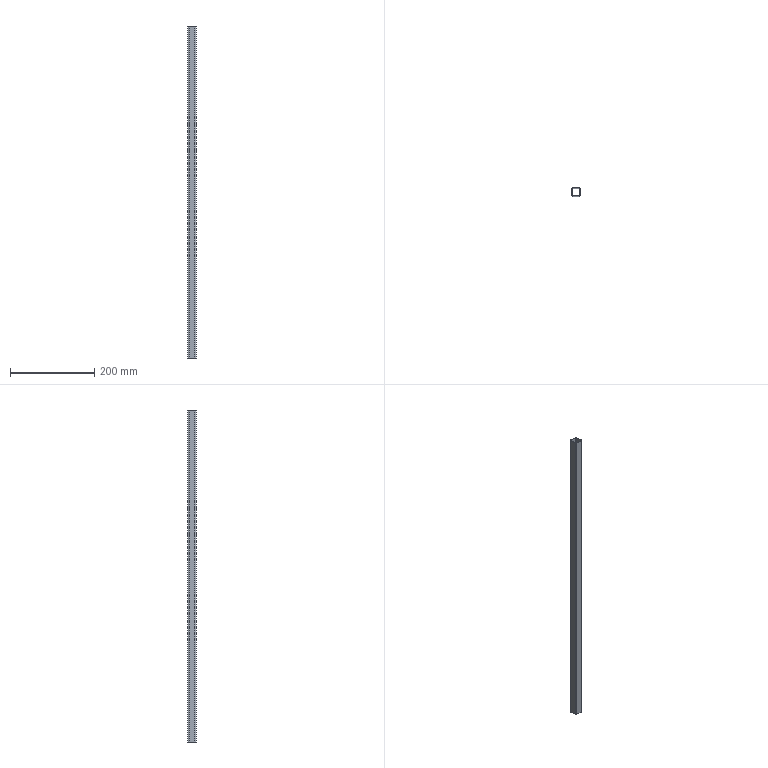Part | SolidWorks | features BaseBody 1 | 1 solid | 18 faces | box 20 x 20 x 786.319 mm | volume 67070 mm3 | plane 10 | cylinder 8 | commonest cylinder face diameters 3.6 x4 6 x4
STEP:
#1=CARTESIAN_POINT('',(7.,-8.8,0.));
#2=VERTEX_POINT('',#1);
#3=CARTESIAN_POINT('',(7.,-8.8,786.319));
#4=VERTEX_POINT('',#3);
#5=CARTESIAN_POINT('',(7.,-8.8,0.));
#6=DIRECTION('',(0.,0.,1.));
#7=VECTOR('',#6,1000.);
#8=LINE('',#5,#7);
#9=EDGE_CURVE('',#2,#4,#8,.T.);
#10=ORIENTED_EDGE('',*,*,#9,.F.);
#11=CARTESIAN_POINT('',(-7.,-8.8,0.));
#12=VERTEX_POINT('',#11);
#13=CARTESIAN_POINT('',(7.,-8.8,0.));
#14=DIRECTION('',(1.,0.,0.));
#15=VECTOR('',#14,1000.);
#16=LINE('',#13,#15);
#17=EDGE_CURVE('',#12,#2,#16,.T.);
#18=ORIENTED_EDGE('',*,*,#17,.F.);
#19=CARTESIAN_POINT('',(-7.,-8.8,786.319));
#20=VERTEX_POINT('',#19);
#21=CARTESIAN_POINT('',(-7.,-8.8,0.));
#22=DIRECTION('',(0.,0.,-1.));
#23=VECTOR('',#22,1000.);
#24=LINE('',#21,#23);
#25=EDGE_CURVE('',#20,#12,#24,.T.);
#26=ORIENTED_EDGE('',*,*,#25,.F.);
#27=CARTESIAN_POINT('',(7.,-8.8,786.319));
#28=DIRECTION('',(-1.,0.,0.));
#29=VECTOR('',#28,1000.);
#30=LINE('',#27,#29);
#31=EDGE_CURVE('',#4,#20,#30,.T.);
#32=ORIENTED_EDGE('',*,*,#31,.F.);
#33=EDGE_LOOP('',(#10,#18,#26,#32));
#34=FACE_OUTER_BOUND('',#33,.T.);
#35=CARTESIAN_POINT('',(7.,-8.8,0.));
#36=DIRECTION('',(0.,-1.,0.));
#37=DIRECTION('',(1.,0.,0.));
#38=AXIS2_PLACEMENT_3D('',#35,#36,#37);
#39=PLANE('',#38);
#40=ADVANCED_FACE('',(#34),#39,.F.);
#41=CARTESIAN_POINT('',(-8.8,-7.,786.319));
#42=VERTEX_POINT('',#41);
#43=CARTESIAN_POINT('',(-8.8,7.,786.319));
#44=VERTEX_POINT('',#43);
#45=CARTESIAN_POINT('',(-8.8,0.,786.319));
#46=DIRECTION('',(0.,1.,0.));
#47=VECTOR('',#46,1000.);
#48=LINE('',#45,#47);
#49=EDGE_CURVE('',#42,#44,#48,.T.);
#50=ORIENTED_EDGE('',*,*,#49,.T.);
#51=CARTESIAN_POINT('',(-7.,8.8,786.319));
#52=VERTEX_POINT('',#51);
#53=CARTESIAN_POINT('',(-7.,7.,786.319));
#54=DIRECTION('',(0.,0.,-1.));
#55=DIRECTION('',(1.,0.,0.));
#56=AXIS2_PLACEMENT_3D('',#53,#54,#55);
#57=CIRCLE('',#56,1.8);
#58=EDGE_CURVE('',#44,#52,#57,.T.);
#59=ORIENTED_EDGE('',*,*,#58,.T.);
#60=CARTESIAN_POINT('',(7.,8.8,786.319));
#61=VERTEX_POINT('',#60);
#62=CARTESIAN_POINT('',(0.,8.8,786.319));
#63=DIRECTION('',(1.,0.,0.));
#64=VECTOR('',#63,1000.);
#65=LINE('',#62,#64);
#66=EDGE_CURVE('',#52,#61,#65,.T.);
#67=ORIENTED_EDGE('',*,*,#66,.T.);
#68=CARTESIAN_POINT('',(8.8,7.,786.319));
#69=VERTEX_POINT('',#68);
#70=CARTESIAN_POINT('',(7.,7.,786.319));
#71=DIRECTION('',(0.,0.,-1.));
#72=DIRECTION('',(1.,0.,0.));
#73=AXIS2_PLACEMENT_3D('',#70,#71,#72);
#74=CIRCLE('',#73,1.8);
#75=EDGE_CURVE('',#61,#69,#74,.T.);
#76=ORIENTED_EDGE('',*,*,#75,.T.);
#77=CARTESIAN_POINT('',(8.8,-7.,786.319));
#78=VERTEX_POINT('',#77);
#79=CARTESIAN_POINT('',(8.8,0.,786.319));
#80=DIRECTION('',(0.,-1.,0.));
#81=VECTOR('',#80,1000.);
#82=LINE('',#79,#81);
#83=EDGE_CURVE('',#69,#78,#82,.T.);
#84=ORIENTED_EDGE('',*,*,#83,.T.);
#85=CARTESIAN_POINT('',(7.,-7.,786.319));
#86=DIRECTION('',(0.,0.,-1.));
#87=DIRECTION('',(1.,0.,0.));
#88=AXIS2_PLACEMENT_3D('',#85,#86,#87);
#89=CIRCLE('',#88,1.8);
#90=EDGE_CURVE('',#78,#4,#89,.T.);
#91=ORIENTED_EDGE('',*,*,#90,.T.);
#92=ORIENTED_EDGE('',*,*,#31,.T.);
#93=CARTESIAN_POINT('',(-7.,-7.,786.319));
#94=DIRECTION('',(0.,0.,-1.));
#95=DIRECTION('',(1.,0.,0.));
#96=AXIS2_PLACEMENT_3D('',#93,#94,#95);
#97=CIRCLE('',#96,1.8);
#98=EDGE_CURVE('',#20,#42,#97,.T.);
#99=ORIENTED_EDGE('',*,*,#98,.T.);
#100=EDGE_LOOP('',(#50,#59,#67,#76,#84,#91,#92,#99));
#101=FACE_BOUND('',#100,.T.);
#102=CARTESIAN_POINT('',(7.,10.,786.319));
#103=VERTEX_POINT('',#102);
#104=CARTESIAN_POINT('',(-7.,10.,786.319));
#105=VERTEX_POINT('',#104);
#106=CARTESIAN_POINT('',(0.,10.,786.319));
#107=DIRECTION('',(-1.,0.,0.));
#108=VECTOR('',#107,1000.);
#109=LINE('',#106,#108);
#110=EDGE_CURVE('',#103,#105,#109,.T.);
#111=ORIENTED_EDGE('',*,*,#110,.T.);
#112=CARTESIAN_POINT('',(-10.,7.,786.319));
#113=VERTEX_POINT('',#112);
#114=CARTESIAN_POINT('',(-7.,7.,786.319));
#115=DIRECTION('',(0.,0.,1.));
#116=DIRECTION('',(1.,0.,0.));
#117=AXIS2_PLACEMENT_3D('',#114,#115,#116);
#118=CIRCLE('',#117,3.);
#119=EDGE_CURVE('',#105,#113,#118,.T.);
#120=ORIENTED_EDGE('',*,*,#119,.T.);
#121=CARTESIAN_POINT('',(-10.,-7.,786.319));
#122=VERTEX_POINT('',#121);
#123=CARTESIAN_POINT('',(-10.,0.,786.319));
#124=DIRECTION('',(0.,-1.,0.));
#125=VECTOR('',#124,1000.);
#126=LINE('',#123,#125);
#127=EDGE_CURVE('',#113,#122,#126,.T.);
#128=ORIENTED_EDGE('',*,*,#127,.T.);
#129=CARTESIAN_POINT('',(-7.,-10.,786.319));
#130=VERTEX_POINT('',#129);
#131=CARTESIAN_POINT('',(-7.,-7.,786.319));
#132=DIRECTION('',(0.,0.,1.));
#133=DIRECTION('',(1.,0.,0.));
#134=AXIS2_PLACEMENT_3D('',#131,#132,#133);
#135=CIRCLE('',#134,3.);
#136=EDGE_CURVE('',#122,#130,#135,.T.);
#137=ORIENTED_EDGE('',*,*,#136,.T.);
#138=CARTESIAN_POINT('',(7.,-10.,786.319));
#139=VERTEX_POINT('',#138);
#140=CARTESIAN_POINT('',(0.,-10.,786.319));
#141=DIRECTION('',(1.,0.,0.));
#142=VECTOR('',#141,1000.);
#143=LINE('',#140,#142);
#144=EDGE_CURVE('',#130,#139,#143,.T.);
#145=ORIENTED_EDGE('',*,*,#144,.T.);
#146=CARTESIAN_POINT('',(10.,-7.,786.319));
#147=VERTEX_POINT('',#146);
#148=CARTESIAN_POINT('',(7.,-7.,786.319));
#149=DIRECTION('',(0.,0.,1.));
#150=DIRECTION('',(1.,0.,0.));
#151=AXIS2_PLACEMENT_3D('',#148,#149,#150);
#152=CIRCLE('',#151,3.);
#153=EDGE_CURVE('',#139,#147,#152,.T.);
#154=ORIENTED_EDGE('',*,*,#153,.T.);
#155=CARTESIAN_POINT('',(10.,7.,786.319));
#156=VERTEX_POINT('',#155);
#157=CARTESIAN_POINT('',(10.,0.,786.319));
#158=DIRECTION('',(0.,1.,0.));
#159=VECTOR('',#158,1000.);
#160=LINE('',#157,#159);
#161=EDGE_CURVE('',#147,#156,#160,.T.);
#162=ORIENTED_EDGE('',*,*,#161,.T.);
#163=CARTESIAN_POINT('',(7.,7.,786.319));
#164=DIRECTION('',(0.,0.,1.));
#165=DIRECTION('',(1.,0.,0.));
#166=AXIS2_PLACEMENT_3D('',#163,#164,#165);
#167=CIRCLE('',#166,3.);
#168=EDGE_CURVE('',#156,#103,#167,.T.);
#169=ORIENTED_EDGE('',*,*,#168,.T.);
#170=EDGE_LOOP('',(#111,#120,#128,#137,#145,#154,#162,#169));
#171=FACE_OUTER_BOUND('',#170,.T.);
#172=CARTESIAN_POINT('',(0.,0.,786.319));
#173=DIRECTION('',(0.,0.,1.));
#174=DIRECTION('',(1.,0.,0.));
#175=AXIS2_PLACEMENT_3D('',#172,#173,#174);
#176=PLANE('',#175);
#177=ADVANCED_FACE('',(#101,#171),#176,.T.);
#178=CARTESIAN_POINT('',(8.8,-7.,0.));
#179=VERTEX_POINT('',#178);
#180=CARTESIAN_POINT('',(8.8,-7.,0.));
#181=DIRECTION('',(0.,0.,1.));
#182=VECTOR('',#181,1000.);
#183=LINE('',#180,#182);
#184=EDGE_CURVE('',#179,#78,#183,.T.);
#185=ORIENTED_EDGE('',*,*,#184,.F.);
#186=CARTESIAN_POINT('',(7.,-7.,0.));
#187=DIRECTION('',(0.,0.,1.));
#188=DIRECTION('',(1.,0.,0.));
#189=AXIS2_PLACEMENT_3D('',#186,#187,#188);
#190=CIRCLE('',#189,1.8);
#191=EDGE_CURVE('',#2,#179,#190,.T.);
#192=ORIENTED_EDGE('',*,*,#191,.F.);
#193=ORIENTED_EDGE('',*,*,#9,.T.);
#194=ORIENTED_EDGE('',*,*,#90,.F.);
#195=EDGE_LOOP('',(#185,#192,#193,#194));
#196=FACE_OUTER_BOUND('',#195,.T.);
#197=CARTESIAN_POINT('',(7.,-7.,0.));
#198=DIRECTION('',(0.,0.,1.));
#199=DIRECTION('',(1.,0.,0.));
#200=AXIS2_PLACEMENT_3D('',#197,#198,#199);
#201=CYLINDRICAL_SURFACE('',#200,1.8);
#202=ADVANCED_FACE('',(#196),#201,.F.);
#203=CARTESIAN_POINT('',(-8.8,7.,0.));
#204=VERTEX_POINT('',#203);
#205=CARTESIAN_POINT('',(-7.,8.8,0.));
#206=VERTEX_POINT('',#205);
#207=CARTESIAN_POINT('',(-7.,7.,0.));
#208=DIRECTION('',(0.,0.,-1.));
#209=DIRECTION('',(1.,0.,0.));
#210=AXIS2_PLACEMENT_3D('',#207,#208,#209);
#211=CIRCLE('',#210,1.8);
#212=EDGE_CURVE('',#204,#206,#211,.T.);
#213=ORIENTED_EDGE('',*,*,#212,.F.);
#214=CARTESIAN_POINT('',(-8.8,-7.,0.));
#215=VERTEX_POINT('',#214);
#216=CARTESIAN_POINT('',(-8.8,0.,0.));
#217=DIRECTION('',(0.,1.,0.));
#218=VECTOR('',#217,1000.);
#219=LINE('',#216,#218);
#220=EDGE_CURVE('',#215,#204,#219,.T.);
#221=ORIENTED_EDGE('',*,*,#220,.F.);
#222=CARTESIAN_POINT('',(-7.,-7.,0.));
#223=DIRECTION('',(0.,0.,-1.));
#224=DIRECTION('',(1.,0.,0.));
#225=AXIS2_PLACEMENT_3D('',#222,#223,#224);
#226=CIRCLE('',#225,1.8);
#227=EDGE_CURVE('',#12,#215,#226,.T.);
#228=ORIENTED_EDGE('',*,*,#227,.F.);
#229=ORIENTED_EDGE('',*,*,#17,.T.);
#230=ORIENTED_EDGE('',*,*,#191,.T.);
#231=CARTESIAN_POINT('',(8.8,7.,0.));
#232=VERTEX_POINT('',#231);
#233=CARTESIAN_POINT('',(8.8,0.,0.));
#234=DIRECTION('',(0.,-1.,0.));
#235=VECTOR('',#234,1000.);
#236=LINE('',#233,#235);
#237=EDGE_CURVE('',#232,#179,#236,.T.);
#238=ORIENTED_EDGE('',*,*,#237,.F.);
#239=CARTESIAN_POINT('',(7.,8.8,0.));
#240=VERTEX_POINT('',#239);
#241=CARTESIAN_POINT('',(7.,7.,0.));
#242=DIRECTION('',(0.,0.,-1.));
#243=DIRECTION('',(1.,0.,0.));
#244=AXIS2_PLACEMENT_3D('',#241,#242,#243);
#245=CIRCLE('',#244,1.8);
#246=EDGE_CURVE('',#240,#232,#245,.T.);
#247=ORIENTED_EDGE('',*,*,#246,.F.);
#248=CARTESIAN_POINT('',(0.,8.8,0.));
#249=DIRECTION('',(1.,0.,0.));
#250=VECTOR('',#249,1000.);
#251=LINE('',#248,#250);
#252=EDGE_CURVE('',#206,#240,#251,.T.);
#253=ORIENTED_EDGE('',*,*,#252,.F.);
#254=EDGE_LOOP('',(#213,#221,#228,#229,#230,#238,#247,#253));
#255=FACE_BOUND('',#254,.T.);
#256=CARTESIAN_POINT('',(-7.,10.,0.));
#257=VERTEX_POINT('',#256);
#258=CARTESIAN_POINT('',(-10.,7.,0.));
#259=VERTEX_POINT('',#258);
#260=CARTESIAN_POINT('',(-7.,7.,0.));
#261=DIRECTION('',(0.,0.,1.));
#262=DIRECTION('',(1.,0.,0.));
#263=AXIS2_PLACEMENT_3D('',#260,#261,#262);
#264=CIRCLE('',#263,3.);
#265=EDGE_CURVE('',#257,#259,#264,.T.);
#266=ORIENTED_EDGE('',*,*,#265,.F.);
#267=CARTESIAN_POINT('',(7.,10.,0.));
#268=VERTEX_POINT('',#267);
#269=CARTESIAN_POINT('',(0.,10.,0.));
#270=DIRECTION('',(-1.,0.,0.));
#271=VECTOR('',#270,1000.);
#272=LINE('',#269,#271);
#273=EDGE_CURVE('',#268,#257,#272,.T.);
#274=ORIENTED_EDGE('',*,*,#273,.F.);
#275=CARTESIAN_POINT('',(10.,7.,0.));
#276=VERTEX_POINT('',#275);
#277=CARTESIAN_POINT('',(7.,7.,0.));
#278=DIRECTION('',(0.,0.,1.));
#279=DIRECTION('',(1.,0.,0.));
#280=AXIS2_PLACEMENT_3D('',#277,#278,#279);
#281=CIRCLE('',#280,3.);
#282=EDGE_CURVE('',#276,#268,#281,.T.);
#283=ORIENTED_EDGE('',*,*,#282,.F.);
#284=CARTESIAN_POINT('',(10.,-7.,0.));
#285=VERTEX_POINT('',#284);
#286=CARTESIAN_POINT('',(10.,0.,0.));
#287=DIRECTION('',(0.,1.,0.));
#288=VECTOR('',#287,1000.);
#289=LINE('',#286,#288);
#290=EDGE_CURVE('',#285,#276,#289,.T.);
#291=ORIENTED_EDGE('',*,*,#290,.F.);
#292=CARTESIAN_POINT('',(7.,-10.,0.));
#293=VERTEX_POINT('',#292);
#294=CARTESIAN_POINT('',(7.,-7.,0.));
#295=DIRECTION('',(0.,0.,1.));
#296=DIRECTION('',(1.,0.,0.));
#297=AXIS2_PLACEMENT_3D('',#294,#295,#296);
#298=CIRCLE('',#297,3.);
#299=EDGE_CURVE('',#293,#285,#298,.T.);
#300=ORIENTED_EDGE('',*,*,#299,.F.);
#301=CARTESIAN_POINT('',(-7.,-10.,0.));
#302=VERTEX_POINT('',#301);
#303=CARTESIAN_POINT('',(0.,-10.,0.));
#304=DIRECTION('',(1.,0.,0.));
#305=VECTOR('',#304,1000.);
#306=LINE('',#303,#305);
#307=EDGE_CURVE('',#302,#293,#306,.T.);
#308=ORIENTED_EDGE('',*,*,#307,.F.);
#309=CARTESIAN_POINT('',(-10.,-7.,0.));
#310=VERTEX_POINT('',#309);
#311=CARTESIAN_POINT('',(-7.,-7.,0.));
#312=DIRECTION('',(0.,0.,1.));
#313=DIRECTION('',(1.,0.,0.));
#314=AXIS2_PLACEMENT_3D('',#311,#312,#313);
#315=CIRCLE('',#314,3.);
#316=EDGE_CURVE('',#310,#302,#315,.T.);
#317=ORIENTED_EDGE('',*,*,#316,.F.);
#318=CARTESIAN_POINT('',(-10.,0.,0.));
#319=DIRECTION('',(0.,-1.,0.));
#320=VECTOR('',#319,1000.);
#321=LINE('',#318,#320);
#322=EDGE_CURVE('',#259,#310,#321,.T.);
#323=ORIENTED_EDGE('',*,*,#322,.F.);
#324=EDGE_LOOP('',(#266,#274,#283,#291,#300,#308,#317,#323));
#325=FACE_OUTER_BOUND('',#324,.T.);
#326=CARTESIAN_POINT('',(0.,0.,0.));
#327=DIRECTION('',(0.,0.,1.));
#328=DIRECTION('',(1.,0.,0.));
#329=AXIS2_PLACEMENT_3D('',#326,#327,#328);
#330=PLANE('',#329);
#331=ADVANCED_FACE('',(#255,#325),#330,.F.);
#332=ORIENTED_EDGE('',*,*,#25,.T.);
#333=ORIENTED_EDGE('',*,*,#227,.T.);
#334=CARTESIAN_POINT('',(-8.8,-7.,0.));
#335=DIRECTION('',(0.,0.,-1.));
#336=VECTOR('',#335,1000.);
#337=LINE('',#334,#336);
#338=EDGE_CURVE('',#42,#215,#337,.T.);
#339=ORIENTED_EDGE('',*,*,#338,.F.);
#340=ORIENTED_EDGE('',*,*,#98,.F.);
#341=EDGE_LOOP('',(#332,#333,#339,#340));
#342=FACE_OUTER_BOUND('',#341,.T.);
#343=CARTESIAN_POINT('',(-7.,-7.,0.));
#344=DIRECTION('',(0.,0.,1.));
#345=DIRECTION('',(1.,0.,0.));
#346=AXIS2_PLACEMENT_3D('',#343,#344,#345);
#347=CYLINDRICAL_SURFACE('',#346,1.8);
#348=ADVANCED_FACE('',(#342),#347,.F.);
#349=CARTESIAN_POINT('',(-8.8,7.,0.));
#350=DIRECTION('',(0.,0.,1.));
#351=VECTOR('',#350,1000.);
#352=LINE('',#349,#351);
#353=EDGE_CURVE('',#204,#44,#352,.T.);
#354=ORIENTED_EDGE('',*,*,#353,.F.);
#355=ORIENTED_EDGE('',*,*,#212,.T.);
#356=CARTESIAN_POINT('',(-7.,8.8,0.));
#357=DIRECTION('',(0.,0.,-1.));
#358=VECTOR('',#357,1000.);
#359=LINE('',#356,#358);
#360=EDGE_CURVE('',#52,#206,#359,.T.);
#361=ORIENTED_EDGE('',*,*,#360,.F.);
#362=ORIENTED_EDGE('',*,*,#58,.F.);
#363=EDGE_LOOP('',(#354,#355,#361,#362));
#364=FACE_OUTER_BOUND('',#363,.T.);
#365=CARTESIAN_POINT('',(-7.,7.,0.));
#366=DIRECTION('',(0.,0.,1.));
#367=DIRECTION('',(1.,0.,0.));
#368=AXIS2_PLACEMENT_3D('',#365,#366,#367);
#369=CYLINDRICAL_SURFACE('',#368,1.8);
#370=ADVANCED_FACE('',(#364),#369,.F.);
#371=ORIENTED_EDGE('',*,*,#338,.T.);
#372=ORIENTED_EDGE('',*,*,#220,.T.);
#373=ORIENTED_EDGE('',*,*,#353,.T.);
#374=ORIENTED_EDGE('',*,*,#49,.F.);
#375=EDGE_LOOP('',(#371,#372,#373,#374));
#376=FACE_OUTER_BOUND('',#375,.T.);
#377=CARTESIAN_POINT('',(-8.8,-7.,0.));
#378=DIRECTION('',(-1.,0.,0.));
#379=DIRECTION('',(0.,-1.,0.));
#380=AXIS2_PLACEMENT_3D('',#377,#378,#379);
#381=PLANE('',#380);
#382=ADVANCED_FACE('',(#376),#381,.F.);
#383=CARTESIAN_POINT('',(8.8,7.,0.));
#384=DIRECTION('',(0.,0.,1.));
#385=VECTOR('',#384,1000.);
#386=LINE('',#383,#385);
#387=EDGE_CURVE('',#232,#69,#386,.T.);
#388=ORIENTED_EDGE('',*,*,#387,.F.);
#389=ORIENTED_EDGE('',*,*,#237,.T.);
#390=ORIENTED_EDGE('',*,*,#184,.T.);
#391=ORIENTED_EDGE('',*,*,#83,.F.);
#392=EDGE_LOOP('',(#388,#389,#390,#391));
#393=FACE_OUTER_BOUND('',#392,.T.);
#394=CARTESIAN_POINT('',(8.8,7.,0.));
#395=DIRECTION('',(1.,0.,0.));
#396=DIRECTION('',(0.,0.,-1.));
#397=AXIS2_PLACEMENT_3D('',#394,#395,#396);
#398=PLANE('',#397);
#399=ADVANCED_FACE('',(#393),#398,.F.);
#400=CARTESIAN_POINT('',(7.,8.8,0.));
#401=DIRECTION('',(0.,0.,1.));
#402=VECTOR('',#401,1000.);
#403=LINE('',#400,#402);
#404=EDGE_CURVE('',#240,#61,#403,.T.);
#405=ORIENTED_EDGE('',*,*,#404,.F.);
#406=ORIENTED_EDGE('',*,*,#246,.T.);
#407=ORIENTED_EDGE('',*,*,#387,.T.);
#408=ORIENTED_EDGE('',*,*,#75,.F.);
#409=EDGE_LOOP('',(#405,#406,#407,#408));
#410=FACE_OUTER_BOUND('',#409,.T.);
#411=CARTESIAN_POINT('',(7.,7.,0.));
#412=DIRECTION('',(0.,0.,1.));
#413=DIRECTION('',(1.,0.,0.));
#414=AXIS2_PLACEMENT_3D('',#411,#412,#413);
#415=CYLINDRICAL_SURFACE('',#414,1.8);
#416=ADVANCED_FACE('',(#410),#415,.F.);
#417=ORIENTED_EDGE('',*,*,#360,.T.);
#418=ORIENTED_EDGE('',*,*,#252,.T.);
#419=ORIENTED_EDGE('',*,*,#404,.T.);
#420=ORIENTED_EDGE('',*,*,#66,.F.);
#421=EDGE_LOOP('',(#417,#418,#419,#420));
#422=FACE_OUTER_BOUND('',#421,.T.);
#423=CARTESIAN_POINT('',(-7.,8.8,0.));
#424=DIRECTION('',(0.,1.,0.));
#425=DIRECTION('',(-1.,0.,0.));
#426=AXIS2_PLACEMENT_3D('',#423,#424,#425);
#427=PLANE('',#426);
#428=ADVANCED_FACE('',(#422),#427,.F.);
#429=ORIENTED_EDGE('',*,*,#265,.T.);
#430=CARTESIAN_POINT('',(-10.,7.,0.));
#431=DIRECTION('',(0.,0.,1.));
#432=VECTOR('',#431,1000.);
#433=LINE('',#430,#432);
#434=EDGE_CURVE('',#259,#113,#433,.T.);
#435=ORIENTED_EDGE('',*,*,#434,.T.);
#436=ORIENTED_EDGE('',*,*,#119,.F.);
#437=CARTESIAN_POINT('',(-7.,10.,0.));
#438=DIRECTION('',(0.,0.,-1.));
#439=VECTOR('',#438,1000.);
#440=LINE('',#437,#439);
#441=EDGE_CURVE('',#105,#257,#440,.T.);
#442=ORIENTED_EDGE('',*,*,#441,.T.);
#443=EDGE_LOOP('',(#429,#435,#436,#442));
#444=FACE_OUTER_BOUND('',#443,.T.);
#445=CARTESIAN_POINT('',(-7.,7.,0.));
#446=DIRECTION('',(0.,0.,1.));
#447=DIRECTION('',(1.,0.,0.));
#448=AXIS2_PLACEMENT_3D('',#445,#446,#447);
#449=CYLINDRICAL_SURFACE('',#448,3.);
#450=ADVANCED_FACE('',(#444),#449,.T.);
#451=ORIENTED_EDGE('',*,*,#273,.T.);
#452=ORIENTED_EDGE('',*,*,#441,.F.);
#453=ORIENTED_EDGE('',*,*,#110,.F.);
#454=CARTESIAN_POINT('',(7.,10.,0.));
#455=DIRECTION('',(0.,0.,-1.));
#456=VECTOR('',#455,1000.);
#457=LINE('',#454,#456);
#458=EDGE_CURVE('',#103,#268,#457,.T.);
#459=ORIENTED_EDGE('',*,*,#458,.T.);
#460=EDGE_LOOP('',(#451,#452,#453,#459));
#461=FACE_OUTER_BOUND('',#460,.T.);
#462=CARTESIAN_POINT('',(-7.,10.,0.));
#463=DIRECTION('',(0.,1.,0.));
#464=DIRECTION('',(-1.,0.,0.));
#465=AXIS2_PLACEMENT_3D('',#462,#463,#464);
#466=PLANE('',#465);
#467=ADVANCED_FACE('',(#461),#466,.T.);
#468=ORIENTED_EDGE('',*,*,#282,.T.);
#469=ORIENTED_EDGE('',*,*,#458,.F.);
#470=ORIENTED_EDGE('',*,*,#168,.F.);
#471=CARTESIAN_POINT('',(10.,7.,0.));
#472=DIRECTION('',(0.,0.,-1.));
#473=VECTOR('',#472,1000.);
#474=LINE('',#471,#473);
#475=EDGE_CURVE('',#156,#276,#474,.T.);
#476=ORIENTED_EDGE('',*,*,#475,.T.);
#477=EDGE_LOOP('',(#468,#469,#470,#476));
#478=FACE_OUTER_BOUND('',#477,.T.);
#479=CARTESIAN_POINT('',(7.,7.,0.));
#480=DIRECTION('',(0.,0.,1.));
#481=DIRECTION('',(1.,0.,0.));
#482=AXIS2_PLACEMENT_3D('',#479,#480,#481);
#483=CYLINDRICAL_SURFACE('',#482,3.);
#484=ADVANCED_FACE('',(#478),#483,.T.);
#485=ORIENTED_EDGE('',*,*,#290,.T.);
#486=ORIENTED_EDGE('',*,*,#475,.F.);
#487=ORIENTED_EDGE('',*,*,#161,.F.);
#488=CARTESIAN_POINT('',(10.,-7.,0.));
#489=DIRECTION('',(0.,0.,-1.));
#490=VECTOR('',#489,1000.);
#491=LINE('',#488,#490);
#492=EDGE_CURVE('',#147,#285,#491,.T.);
#493=ORIENTED_EDGE('',*,*,#492,.T.);
#494=EDGE_LOOP('',(#485,#486,#487,#493));
#495=FACE_OUTER_BOUND('',#494,.T.);
#496=CARTESIAN_POINT('',(10.,7.,0.));
#497=DIRECTION('',(1.,0.,0.));
#498=DIRECTION('',(0.,0.,-1.));
#499=AXIS2_PLACEMENT_3D('',#496,#497,#498);
#500=PLANE('',#499);
#501=ADVANCED_FACE('',(#495),#500,.T.);
#502=ORIENTED_EDGE('',*,*,#299,.T.);
#503=ORIENTED_EDGE('',*,*,#492,.F.);
#504=ORIENTED_EDGE('',*,*,#153,.F.);
#505=CARTESIAN_POINT('',(7.,-10.,0.));
#506=DIRECTION('',(0.,0.,-1.));
#507=VECTOR('',#506,1000.);
#508=LINE('',#505,#507);
#509=EDGE_CURVE('',#139,#293,#508,.T.);
#510=ORIENTED_EDGE('',*,*,#509,.T.);
#511=EDGE_LOOP('',(#502,#503,#504,#510));
#512=FACE_OUTER_BOUND('',#511,.T.);
#513=CARTESIAN_POINT('',(7.,-7.,0.));
#514=DIRECTION('',(0.,0.,1.));
#515=DIRECTION('',(1.,0.,0.));
#516=AXIS2_PLACEMENT_3D('',#513,#514,#515);
#517=CYLINDRICAL_SURFACE('',#516,3.);
#518=ADVANCED_FACE('',(#512),#517,.T.);
#519=ORIENTED_EDGE('',*,*,#307,.T.);
#520=ORIENTED_EDGE('',*,*,#509,.F.);
#521=ORIENTED_EDGE('',*,*,#144,.F.);
#522=CARTESIAN_POINT('',(-7.,-10.,0.));
#523=DIRECTION('',(0.,0.,-1.));
#524=VECTOR('',#523,1000.);
#525=LINE('',#522,#524);
#526=EDGE_CURVE('',#130,#302,#525,.T.);
#527=ORIENTED_EDGE('',*,*,#526,.T.);
#528=EDGE_LOOP('',(#519,#520,#521,#527));
#529=FACE_OUTER_BOUND('',#528,.T.);
#530=CARTESIAN_POINT('',(7.,-10.,0.));
#531=DIRECTION('',(0.,-1.,0.));
#532=DIRECTION('',(1.,0.,0.));
#533=AXIS2_PLACEMENT_3D('',#530,#531,#532);
#534=PLANE('',#533);
#535=ADVANCED_FACE('',(#529),#534,.T.);
#536=ORIENTED_EDGE('',*,*,#316,.T.);
#537=ORIENTED_EDGE('',*,*,#526,.F.);
#538=ORIENTED_EDGE('',*,*,#136,.F.);
#539=CARTESIAN_POINT('',(-10.,-7.,0.));
#540=DIRECTION('',(0.,0.,-1.));
#541=VECTOR('',#540,1000.);
#542=LINE('',#539,#541);
#543=EDGE_CURVE('',#122,#310,#542,.T.);
#544=ORIENTED_EDGE('',*,*,#543,.T.);
#545=EDGE_LOOP('',(#536,#537,#538,#544));
#546=FACE_OUTER_BOUND('',#545,.T.);
#547=CARTESIAN_POINT('',(-7.,-7.,0.));
#548=DIRECTION('',(0.,0.,1.));
#549=DIRECTION('',(1.,0.,0.));
#550=AXIS2_PLACEMENT_3D('',#547,#548,#549);
#551=CYLINDRICAL_SURFACE('',#550,3.);
#552=ADVANCED_FACE('',(#546),#551,.T.);
#553=ORIENTED_EDGE('',*,*,#322,.T.);
#554=ORIENTED_EDGE('',*,*,#543,.F.);
#555=ORIENTED_EDGE('',*,*,#127,.F.);
#556=ORIENTED_EDGE('',*,*,#434,.F.);
#557=EDGE_LOOP('',(#553,#554,#555,#556));
#558=FACE_OUTER_BOUND('',#557,.T.);
#559=CARTESIAN_POINT('',(-10.,-7.,0.));
#560=DIRECTION('',(-1.,0.,0.));
#561=DIRECTION('',(0.,-1.,0.));
#562=AXIS2_PLACEMENT_3D('',#559,#560,#561);
#563=PLANE('',#562);
#564=ADVANCED_FACE('',(#558),#563,.T.);
#565=CLOSED_SHELL('',(#40,#177,#202,#331,#348,#370,#382,#399,#416,#428,#450,#467,#484,#501,#518,#535,#552,#564));
#566=MANIFOLD_SOLID_BREP('',#565);
#567=CARTESIAN_POINT('',(0.,0.,0.));
#568=DIRECTION('',(0.,0.,1.));
#569=DIRECTION('',(1.,0.,0.));
#570=AXIS2_PLACEMENT_3D('',#567,#568,#569);
#571=(LENGTH_UNIT()NAMED_UNIT(*)SI_UNIT(.MILLI.,.METRE.));
#572=UNCERTAINTY_MEASURE_WITH_UNIT(LENGTH_MEASURE(0.00001),#571,'','');
#573=(NAMED_UNIT(*)PLANE_ANGLE_UNIT()SI_UNIT($,.RADIAN.));
#574=(NAMED_UNIT(*)SI_UNIT($,.STERADIAN.)SOLID_ANGLE_UNIT());
#575=(GEOMETRIC_REPRESENTATION_CONTEXT(3)GLOBAL_UNCERTAINTY_ASSIGNED_CONTEXT((#572))GLOBAL_UNIT_ASSIGNED_CONTEXT((#571,#573,#574))REPRESENTATION_CONTEXT('',''));
#576=ADVANCED_BREP_SHAPE_REPRESENTATION('',(#566,#570),#575);